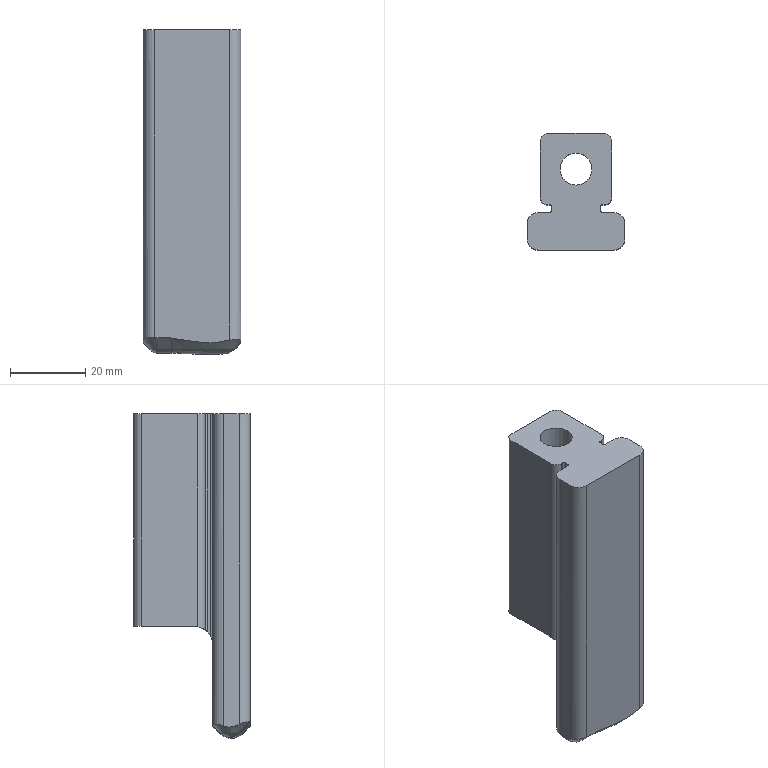Part | NX | features PU-1 2 | 1 solid | 39 faces | box 26 x 31.011 x 86.306 mm | volume 36658 mm3 | cylinder 15 | plane 14 | spline 10 | commonest cylinder face diameters 1 x4 4 x4 6 x4 8.506 x1 10 x1 14.5 x1